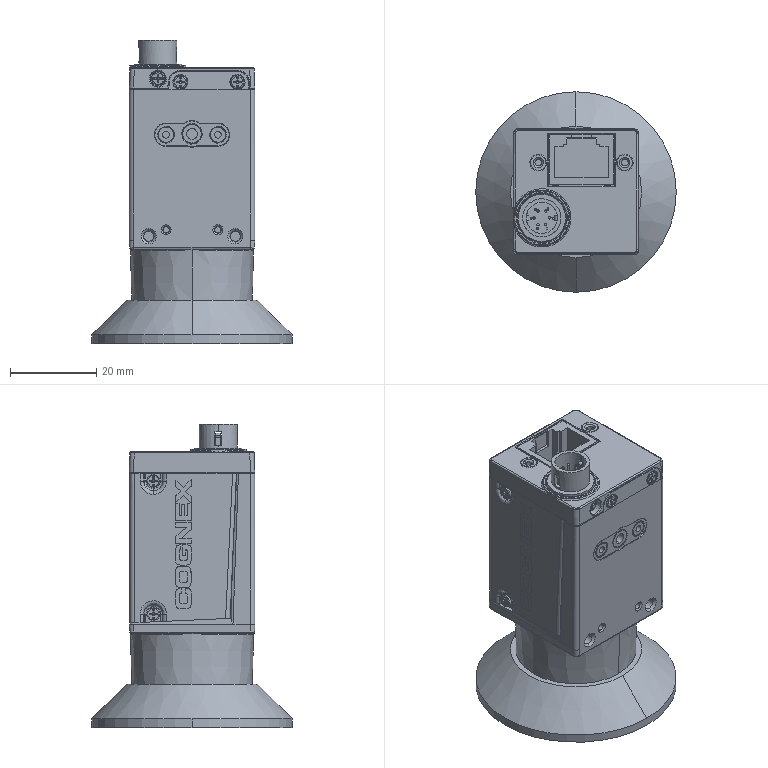Part | SolidWorks | features BaseBody 15 | 15 solids | 1181 faces | box 46.38 x 46.38 x 70.1 mm | volume 45719 mm3 | plane 436 | spline 362 | cylinder 204 | cone 179 | commonest cylinder face diameters 2 x22 3 x18 0.55 x12 0.8 x12 0.814 x12 1.567 x12